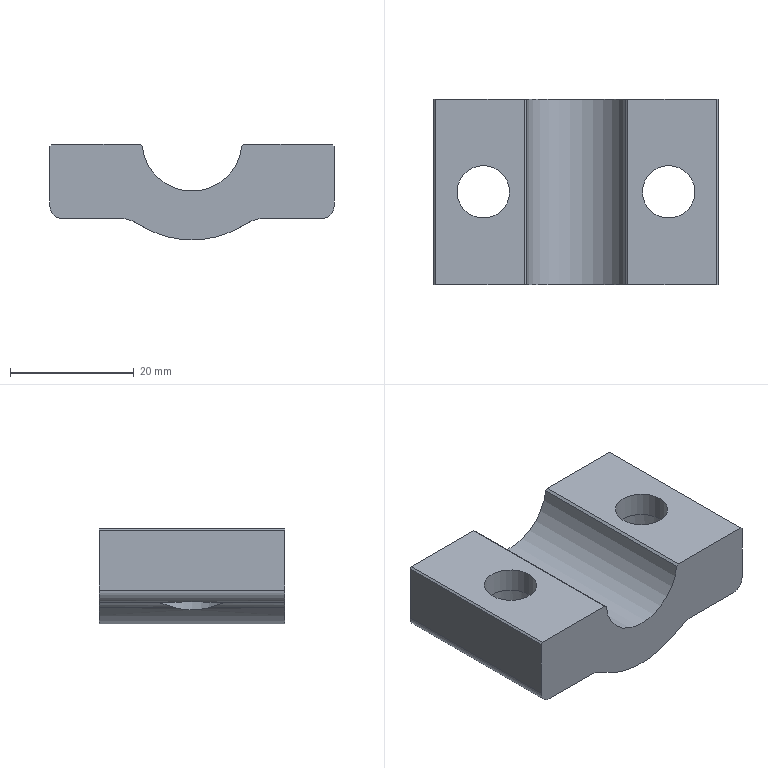Part | NX | 1 solid | 28 faces | box 46 x 30 x 15.5 mm | volume 12341 mm3 | plane 16 | cylinder 12 | commonest cylinder face diameters 10 x4 4 x2 8.5 x2 13.5 x2 16.2 x1 32 x1
STEP:
#1=CARTESIAN_POINT('',(14.61,0.,12.));
#2=VERTEX_POINT('',#1);
#3=CARTESIAN_POINT('',(0.3,0.,12.));
#4=VERTEX_POINT('',#3);
#5=CARTESIAN_POINT('',(23.,0.,12.));
#6=DIRECTION('',(-1.,0.,0.));
#7=VECTOR('',#6,1000.);
#8=LINE('',#5,#7);
#9=EDGE_CURVE('',#2,#4,#8,.T.);
#10=ORIENTED_EDGE('',*,*,#9,.F.);
#11=CARTESIAN_POINT('',(14.61,30.,12.));
#12=VERTEX_POINT('',#11);
#13=CARTESIAN_POINT('',(14.61,30.,12.));
#14=DIRECTION('',(0.,1.,0.));
#15=VECTOR('',#14,1000.);
#16=LINE('',#13,#15);
#17=EDGE_CURVE('',#2,#12,#16,.T.);
#18=ORIENTED_EDGE('',*,*,#17,.T.);
#19=CARTESIAN_POINT('',(0.3,30.,12.));
#20=VERTEX_POINT('',#19);
#21=CARTESIAN_POINT('',(23.,30.,12.));
#22=DIRECTION('',(1.,0.,0.));
#23=VECTOR('',#22,1000.);
#24=LINE('',#21,#23);
#25=EDGE_CURVE('',#20,#12,#24,.T.);
#26=ORIENTED_EDGE('',*,*,#25,.F.);
#27=CARTESIAN_POINT('',(0.3,15.,12.));
#28=DIRECTION('',(0.,-1.,0.));
#29=VECTOR('',#28,1000.);
#30=LINE('',#27,#29);
#31=EDGE_CURVE('',#20,#4,#30,.T.);
#32=ORIENTED_EDGE('',*,*,#31,.T.);
#33=EDGE_LOOP('',(#10,#18,#26,#32));
#34=FACE_BOUND('',#33,.T.);
#35=CARTESIAN_POINT('',(12.25,15.,12.));
#36=VERTEX_POINT('',#35);
#37=CARTESIAN_POINT('',(8.,15.,12.));
#38=DIRECTION('',(0.,0.,-1.));
#39=DIRECTION('',(1.,0.,0.));
#40=AXIS2_PLACEMENT_3D('',#37,#38,#39);
#41=CIRCLE('',#40,4.25);
#42=EDGE_CURVE('',#36,#36,#41,.T.);
#43=ORIENTED_EDGE('',*,*,#42,.T.);
#44=EDGE_LOOP('',(#43));
#45=FACE_BOUND('',#44,.T.);
#46=CARTESIAN_POINT('',(23.,15.,12.));
#47=DIRECTION('',(0.,0.,1.));
#48=DIRECTION('',(1.,0.,0.));
#49=AXIS2_PLACEMENT_3D('',#46,#47,#48);
#50=PLANE('',#49);
#51=ADVANCED_FACE('',(#34,#45),#50,.T.);
#52=CARTESIAN_POINT('',(34.608,0.,0.));
#53=VERTEX_POINT('',#52);
#54=CARTESIAN_POINT('',(34.608,9.164,0.));
#55=VERTEX_POINT('',#54);
#56=CARTESIAN_POINT('',(34.608,30.,0.));
#57=DIRECTION('',(0.,1.,0.));
#58=VECTOR('',#57,1000.);
#59=LINE('',#56,#58);
#60=EDGE_CURVE('',#53,#55,#59,.T.);
#61=ORIENTED_EDGE('',*,*,#60,.T.);
#62=CARTESIAN_POINT('',(44.,11.908,0.));
#63=VERTEX_POINT('',#62);
#64=CARTESIAN_POINT('',(38.,15.,0.));
#65=DIRECTION('',(0.,0.,-1.));
#66=DIRECTION('',(-1.,0.,0.));
#67=AXIS2_PLACEMENT_3D('',#64,#65,#66);
#68=CIRCLE('',#67,6.75);
#69=EDGE_CURVE('',#55,#63,#68,.F.);
#70=ORIENTED_EDGE('',*,*,#69,.T.);
#71=CARTESIAN_POINT('',(44.,0.,0.));
#72=VERTEX_POINT('',#71);
#73=CARTESIAN_POINT('',(44.,15.,0.));
#74=DIRECTION('',(0.,1.,0.));
#75=VECTOR('',#74,1000.);
#76=LINE('',#73,#75);
#77=EDGE_CURVE('',#63,#72,#76,.F.);
#78=ORIENTED_EDGE('',*,*,#77,.T.);
#79=CARTESIAN_POINT('',(23.,0.,0.));
#80=DIRECTION('',(1.,0.,0.));
#81=VECTOR('',#80,1000.);
#82=LINE('',#79,#81);
#83=EDGE_CURVE('',#53,#72,#82,.T.);
#84=ORIENTED_EDGE('',*,*,#83,.F.);
#85=EDGE_LOOP('',(#61,#70,#78,#84));
#86=FACE_BOUND('',#85,.T.);
#87=CARTESIAN_POINT('',(23.,15.,0.));
#88=DIRECTION('',(0.,0.,-1.));
#89=DIRECTION('',(-1.,0.,0.));
#90=AXIS2_PLACEMENT_3D('',#87,#88,#89);
#91=PLANE('',#90);
#92=ADVANCED_FACE('',(#86),#91,.T.);
#93=CARTESIAN_POINT('',(2.,0.,0.));
#94=VERTEX_POINT('',#93);
#95=CARTESIAN_POINT('',(2.,11.908,0.));
#96=VERTEX_POINT('',#95);
#97=CARTESIAN_POINT('',(2.,15.,0.));
#98=DIRECTION('',(0.,-1.,0.));
#99=VECTOR('',#98,1000.);
#100=LINE('',#97,#99);
#101=EDGE_CURVE('',#94,#96,#100,.F.);
#102=ORIENTED_EDGE('',*,*,#101,.T.);
#103=CARTESIAN_POINT('',(11.392,9.164,0.));
#104=VERTEX_POINT('',#103);
#105=CARTESIAN_POINT('',(8.,15.,0.));
#106=DIRECTION('',(0.,0.,-1.));
#107=DIRECTION('',(-1.,0.,0.));
#108=AXIS2_PLACEMENT_3D('',#105,#106,#107);
#109=CIRCLE('',#108,6.75);
#110=EDGE_CURVE('',#96,#104,#109,.F.);
#111=ORIENTED_EDGE('',*,*,#110,.T.);
#112=CARTESIAN_POINT('',(11.392,0.,0.));
#113=VERTEX_POINT('',#112);
#114=CARTESIAN_POINT('',(11.392,0.,0.));
#115=DIRECTION('',(0.,1.,0.));
#116=VECTOR('',#115,1000.);
#117=LINE('',#114,#116);
#118=EDGE_CURVE('',#104,#113,#117,.F.);
#119=ORIENTED_EDGE('',*,*,#118,.T.);
#120=CARTESIAN_POINT('',(23.,0.,0.));
#121=DIRECTION('',(1.,0.,0.));
#122=VECTOR('',#121,1000.);
#123=LINE('',#120,#122);
#124=EDGE_CURVE('',#94,#113,#123,.T.);
#125=ORIENTED_EDGE('',*,*,#124,.F.);
#126=EDGE_LOOP('',(#102,#111,#119,#125));
#127=FACE_BOUND('',#126,.T.);
#128=CARTESIAN_POINT('',(23.,15.,0.));
#129=DIRECTION('',(0.,0.,-1.));
#130=DIRECTION('',(-1.,0.,0.));
#131=AXIS2_PLACEMENT_3D('',#128,#129,#130);
#132=PLANE('',#131);
#133=ADVANCED_FACE('',(#127),#132,.T.);
#134=CARTESIAN_POINT('',(14.156,0.,-0.8333));
#135=VERTEX_POINT('',#134);
#136=CARTESIAN_POINT('',(14.156,12.23,-0.8333));
#137=VERTEX_POINT('',#136);
#138=CARTESIAN_POINT('',(14.156,30.,-0.8333));
#139=DIRECTION('',(0.,-1.,0.));
#140=VECTOR('',#139,1000.);
#141=LINE('',#138,#140);
#142=EDGE_CURVE('',#135,#137,#141,.F.);
#143=ORIENTED_EDGE('',*,*,#142,.T.);
#144=CARTESIAN_POINT('',(14.156,17.77,-0.8333));
#145=VERTEX_POINT('',#144);
#146=CARTESIAN_POINT('',(14.156,12.23,-0.8333));
#147=CARTESIAN_POINT('',(14.925,13.939,-1.343));
#148=CARTESIAN_POINT('',(14.925,16.061,-1.343));
#149=CARTESIAN_POINT('',(14.156,17.77,-0.8333));
#150=B_SPLINE_CURVE_WITH_KNOTS('',3,(#146,#147,#148,#149),.UNSPECIFIED.,.F.,.F.,(4,4),(0.,0.005745),.UNSPECIFIED.);
#151=EDGE_CURVE('',#137,#145,#150,.T.);
#152=ORIENTED_EDGE('',*,*,#151,.T.);
#153=CARTESIAN_POINT('',(14.156,30.,-0.8333));
#154=VERTEX_POINT('',#153);
#155=CARTESIAN_POINT('',(14.156,30.,-0.8333));
#156=DIRECTION('',(0.,-1.,0.));
#157=VECTOR('',#156,1000.);
#158=LINE('',#155,#157);
#159=EDGE_CURVE('',#145,#154,#158,.F.);
#160=ORIENTED_EDGE('',*,*,#159,.T.);
#161=CARTESIAN_POINT('',(31.844,30.,-0.8333));
#162=VERTEX_POINT('',#161);
#163=CARTESIAN_POINT('',(23.,30.,12.5));
#164=DIRECTION('',(0.,-1.,0.));
#165=DIRECTION('',(1.,0.,0.));
#166=AXIS2_PLACEMENT_3D('',#163,#164,#165);
#167=CIRCLE('',#166,16.);
#168=EDGE_CURVE('',#154,#162,#167,.T.);
#169=ORIENTED_EDGE('',*,*,#168,.T.);
#170=CARTESIAN_POINT('',(31.844,17.77,-0.8333));
#171=VERTEX_POINT('',#170);
#172=CARTESIAN_POINT('',(31.844,30.,-0.8333));
#173=DIRECTION('',(0.,-1.,0.));
#174=VECTOR('',#173,1000.);
#175=LINE('',#172,#174);
#176=EDGE_CURVE('',#162,#171,#175,.T.);
#177=ORIENTED_EDGE('',*,*,#176,.T.);
#178=CARTESIAN_POINT('',(31.844,12.23,-0.8333));
#179=VERTEX_POINT('',#178);
#180=CARTESIAN_POINT('',(31.844,17.77,-0.8333));
#181=CARTESIAN_POINT('',(31.075,16.061,-1.343));
#182=CARTESIAN_POINT('',(31.075,13.939,-1.343));
#183=CARTESIAN_POINT('',(31.844,12.23,-0.8333));
#184=B_SPLINE_CURVE_WITH_KNOTS('',3,(#180,#181,#182,#183),.UNSPECIFIED.,.F.,.F.,(4,4),(0.,0.005745),.UNSPECIFIED.);
#185=EDGE_CURVE('',#171,#179,#184,.T.);
#186=ORIENTED_EDGE('',*,*,#185,.T.);
#187=CARTESIAN_POINT('',(31.844,0.,-0.8333));
#188=VERTEX_POINT('',#187);
#189=CARTESIAN_POINT('',(31.844,30.,-0.8333));
#190=DIRECTION('',(0.,-1.,0.));
#191=VECTOR('',#190,1000.);
#192=LINE('',#189,#191);
#193=EDGE_CURVE('',#179,#188,#192,.T.);
#194=ORIENTED_EDGE('',*,*,#193,.T.);
#195=CARTESIAN_POINT('',(23.,0.,12.5));
#196=DIRECTION('',(0.,1.,0.));
#197=DIRECTION('',(1.,0.,0.));
#198=AXIS2_PLACEMENT_3D('',#195,#196,#197);
#199=CIRCLE('',#198,16.);
#200=EDGE_CURVE('',#188,#135,#199,.T.);
#201=ORIENTED_EDGE('',*,*,#200,.T.);
#202=EDGE_LOOP('',(#143,#152,#160,#169,#177,#186,#194,#201));
#203=FACE_BOUND('',#202,.T.);
#204=CARTESIAN_POINT('',(23.,30.,12.5));
#205=DIRECTION('',(0.,-1.,0.));
#206=DIRECTION('',(1.,0.,0.));
#207=AXIS2_PLACEMENT_3D('',#204,#205,#206);
#208=CYLINDRICAL_SURFACE('',#207,16.);
#209=ADVANCED_FACE('',(#203),#208,.T.);
#210=CARTESIAN_POINT('',(11.392,20.836,0.));
#211=VERTEX_POINT('',#210);
#212=CARTESIAN_POINT('',(11.392,20.836,0.));
#213=CARTESIAN_POINT('',(12.644,20.108,0.));
#214=CARTESIAN_POINT('',(13.585,19.039,-0.4545));
#215=CARTESIAN_POINT('',(14.156,17.77,-0.8333));
#216=B_SPLINE_CURVE_WITH_KNOTS('',3,(#212,#213,#214,#215),.UNSPECIFIED.,.F.,.F.,(4,4),(0.,0.004272),.UNSPECIFIED.);
#217=EDGE_CURVE('',#211,#145,#216,.T.);
#218=ORIENTED_EDGE('',*,*,#217,.F.);
#219=CARTESIAN_POINT('',(11.392,30.,0.));
#220=VERTEX_POINT('',#219);
#221=CARTESIAN_POINT('',(11.392,0.,0.));
#222=DIRECTION('',(0.,1.,0.));
#223=VECTOR('',#222,1000.);
#224=LINE('',#221,#223);
#225=EDGE_CURVE('',#220,#211,#224,.F.);
#226=ORIENTED_EDGE('',*,*,#225,.F.);
#227=CARTESIAN_POINT('',(11.392,30.,-5.));
#228=DIRECTION('',(0.,1.,0.));
#229=DIRECTION('',(0.,0.,1.));
#230=AXIS2_PLACEMENT_3D('',#227,#228,#229);
#231=CIRCLE('',#230,5.);
#232=EDGE_CURVE('',#154,#220,#231,.F.);
#233=ORIENTED_EDGE('',*,*,#232,.F.);
#234=ORIENTED_EDGE('',*,*,#159,.F.);
#235=EDGE_LOOP('',(#218,#226,#233,#234));
#236=FACE_BOUND('',#235,.T.);
#237=CARTESIAN_POINT('',(11.392,30.,-5.));
#238=DIRECTION('',(0.,-1.,0.));
#239=DIRECTION('',(0.,0.,-1.));
#240=AXIS2_PLACEMENT_3D('',#237,#238,#239);
#241=CYLINDRICAL_SURFACE('',#240,5.);
#242=ADVANCED_FACE('',(#236),#241,.F.);
#243=CARTESIAN_POINT('',(14.156,12.23,-0.8333));
#244=CARTESIAN_POINT('',(13.585,10.961,-0.4545));
#245=CARTESIAN_POINT('',(12.644,9.892,0.));
#246=CARTESIAN_POINT('',(11.392,9.164,0.));
#247=B_SPLINE_CURVE_WITH_KNOTS('',3,(#243,#244,#245,#246),.UNSPECIFIED.,.F.,.F.,(4,4),(0.,0.00426),.UNSPECIFIED.);
#248=EDGE_CURVE('',#137,#104,#247,.T.);
#249=ORIENTED_EDGE('',*,*,#248,.F.);
#250=ORIENTED_EDGE('',*,*,#142,.F.);
#251=CARTESIAN_POINT('',(11.392,0.,-5.));
#252=DIRECTION('',(0.,-1.,0.));
#253=DIRECTION('',(0.,0.,-1.));
#254=AXIS2_PLACEMENT_3D('',#251,#252,#253);
#255=CIRCLE('',#254,5.);
#256=EDGE_CURVE('',#113,#135,#255,.F.);
#257=ORIENTED_EDGE('',*,*,#256,.F.);
#258=ORIENTED_EDGE('',*,*,#118,.F.);
#259=EDGE_LOOP('',(#249,#250,#257,#258));
#260=FACE_BOUND('',#259,.T.);
#261=CARTESIAN_POINT('',(11.392,30.,-5.));
#262=DIRECTION('',(0.,-1.,0.));
#263=DIRECTION('',(0.,0.,-1.));
#264=AXIS2_PLACEMENT_3D('',#261,#262,#263);
#265=CYLINDRICAL_SURFACE('',#264,5.);
#266=ADVANCED_FACE('',(#260),#265,.F.);
#267=CARTESIAN_POINT('',(34.608,20.836,0.));
#268=VERTEX_POINT('',#267);
#269=CARTESIAN_POINT('',(31.844,17.77,-0.8333));
#270=CARTESIAN_POINT('',(32.415,19.039,-0.4545));
#271=CARTESIAN_POINT('',(33.356,20.108,0.));
#272=CARTESIAN_POINT('',(34.608,20.836,0.));
#273=B_SPLINE_CURVE_WITH_KNOTS('',3,(#269,#270,#271,#272),.UNSPECIFIED.,.F.,.F.,(4,4),(0.,0.00426),.UNSPECIFIED.);
#274=EDGE_CURVE('',#171,#268,#273,.T.);
#275=ORIENTED_EDGE('',*,*,#274,.F.);
#276=ORIENTED_EDGE('',*,*,#176,.F.);
#277=CARTESIAN_POINT('',(34.608,30.,0.));
#278=VERTEX_POINT('',#277);
#279=CARTESIAN_POINT('',(34.608,30.,-5.));
#280=DIRECTION('',(0.,1.,0.));
#281=DIRECTION('',(0.,0.,1.));
#282=AXIS2_PLACEMENT_3D('',#279,#280,#281);
#283=CIRCLE('',#282,5.);
#284=EDGE_CURVE('',#278,#162,#283,.F.);
#285=ORIENTED_EDGE('',*,*,#284,.F.);
#286=CARTESIAN_POINT('',(34.608,30.,0.));
#287=DIRECTION('',(0.,1.,0.));
#288=VECTOR('',#287,1000.);
#289=LINE('',#286,#288);
#290=EDGE_CURVE('',#268,#278,#289,.T.);
#291=ORIENTED_EDGE('',*,*,#290,.F.);
#292=EDGE_LOOP('',(#275,#276,#285,#291));
#293=FACE_BOUND('',#292,.T.);
#294=CARTESIAN_POINT('',(34.608,30.,-5.));
#295=DIRECTION('',(0.,-1.,0.));
#296=DIRECTION('',(0.,0.,-1.));
#297=AXIS2_PLACEMENT_3D('',#294,#295,#296);
#298=CYLINDRICAL_SURFACE('',#297,5.);
#299=ADVANCED_FACE('',(#293),#298,.F.);
#300=CARTESIAN_POINT('',(34.608,9.164,0.));
#301=CARTESIAN_POINT('',(33.356,9.892,0.));
#302=CARTESIAN_POINT('',(32.415,10.961,-0.4545));
#303=CARTESIAN_POINT('',(31.844,12.23,-0.8333));
#304=B_SPLINE_CURVE_WITH_KNOTS('',3,(#300,#301,#302,#303),.UNSPECIFIED.,.F.,.F.,(4,4),(0.,0.004272),.UNSPECIFIED.);
#305=EDGE_CURVE('',#55,#179,#304,.T.);
#306=ORIENTED_EDGE('',*,*,#305,.F.);
#307=ORIENTED_EDGE('',*,*,#60,.F.);
#308=CARTESIAN_POINT('',(34.608,0.,-5.));
#309=DIRECTION('',(0.,-1.,0.));
#310=DIRECTION('',(0.,0.,-1.));
#311=AXIS2_PLACEMENT_3D('',#308,#309,#310);
#312=CIRCLE('',#311,5.);
#313=EDGE_CURVE('',#188,#53,#312,.F.);
#314=ORIENTED_EDGE('',*,*,#313,.F.);
#315=ORIENTED_EDGE('',*,*,#193,.F.);
#316=EDGE_LOOP('',(#306,#307,#314,#315));
#317=FACE_BOUND('',#316,.T.);
#318=CARTESIAN_POINT('',(34.608,30.,-5.));
#319=DIRECTION('',(0.,-1.,0.));
#320=DIRECTION('',(0.,0.,-1.));
#321=AXIS2_PLACEMENT_3D('',#318,#319,#320);
#322=CYLINDRICAL_SURFACE('',#321,5.);
#323=ADVANCED_FACE('',(#317),#322,.F.);
#324=ORIENTED_EDGE('',*,*,#77,.F.);
#325=CARTESIAN_POINT('',(44.,18.092,0.));
#326=VERTEX_POINT('',#325);
#327=CARTESIAN_POINT('',(44.,11.908,0.));
#328=CARTESIAN_POINT('',(44.496,12.87,0.));
#329=CARTESIAN_POINT('',(45.004,15.001,0.2919));
#330=CARTESIAN_POINT('',(44.496,17.13,0.));
#331=CARTESIAN_POINT('',(44.,18.092,0.));
#332=B_SPLINE_CURVE_WITH_KNOTS('',3,(#327,#328,#329,#330,#331),.UNSPECIFIED.,.F.,.F.,(4,1,4),(0.,0.003207,0.006415),.UNSPECIFIED.);
#333=EDGE_CURVE('',#63,#326,#332,.T.);
#334=ORIENTED_EDGE('',*,*,#333,.T.);
#335=CARTESIAN_POINT('',(44.,30.,0.));
#336=VERTEX_POINT('',#335);
#337=CARTESIAN_POINT('',(44.,15.,0.));
#338=DIRECTION('',(0.,1.,0.));
#339=VECTOR('',#338,1000.);
#340=LINE('',#337,#339);
#341=EDGE_CURVE('',#336,#326,#340,.F.);
#342=ORIENTED_EDGE('',*,*,#341,.F.);
#343=CARTESIAN_POINT('',(46.,30.,2.));
#344=VERTEX_POINT('',#343);
#345=CARTESIAN_POINT('',(44.,30.,2.));
#346=DIRECTION('',(0.,1.,0.));
#347=DIRECTION('',(0.,0.,1.));
#348=AXIS2_PLACEMENT_3D('',#345,#346,#347);
#349=CIRCLE('',#348,2.);
#350=EDGE_CURVE('',#344,#336,#349,.T.);
#351=ORIENTED_EDGE('',*,*,#350,.F.);
#352=CARTESIAN_POINT('',(46.,0.,2.));
#353=VERTEX_POINT('',#352);
#354=CARTESIAN_POINT('',(46.,15.,2.));
#355=DIRECTION('',(0.,1.,0.));
#356=VECTOR('',#355,1000.);
#357=LINE('',#354,#356);
#358=EDGE_CURVE('',#353,#344,#357,.T.);
#359=ORIENTED_EDGE('',*,*,#358,.F.);
#360=CARTESIAN_POINT('',(44.,0.,2.));
#361=DIRECTION('',(0.,-1.,0.));
#362=DIRECTION('',(0.,0.,-1.));
#363=AXIS2_PLACEMENT_3D('',#360,#361,#362);
#364=CIRCLE('',#363,2.);
#365=EDGE_CURVE('',#72,#353,#364,.T.);
#366=ORIENTED_EDGE('',*,*,#365,.F.);
#367=EDGE_LOOP('',(#324,#334,#342,#351,#359,#366));
#368=FACE_BOUND('',#367,.T.);
#369=CARTESIAN_POINT('',(44.,15.,2.));
#370=DIRECTION('',(0.,1.,0.));
#371=DIRECTION('',(0.,0.,1.));
#372=AXIS2_PLACEMENT_3D('',#369,#370,#371);
#373=CYLINDRICAL_SURFACE('',#372,2.);
#374=ADVANCED_FACE('',(#368),#373,.T.);
#375=CARTESIAN_POINT('',(2.,18.092,0.));
#376=VERTEX_POINT('',#375);
#377=CARTESIAN_POINT('',(2.,30.,0.));
#378=VERTEX_POINT('',#377);
#379=CARTESIAN_POINT('',(2.,15.,0.));
#380=DIRECTION('',(0.,-1.,0.));
#381=VECTOR('',#380,1000.);
#382=LINE('',#379,#381);
#383=EDGE_CURVE('',#376,#378,#382,.F.);
#384=ORIENTED_EDGE('',*,*,#383,.F.);
#385=CARTESIAN_POINT('',(2.,18.092,0.));
#386=CARTESIAN_POINT('',(1.504,17.13,0.));
#387=CARTESIAN_POINT('',(0.9961,14.999,0.2919));
#388=CARTESIAN_POINT('',(1.504,12.87,0.));
#389=CARTESIAN_POINT('',(2.,11.908,0.));
#390=B_SPLINE_CURVE_WITH_KNOTS('',3,(#385,#386,#387,#388,#389),.UNSPECIFIED.,.F.,.F.,(4,1,4),(0.,0.003207,0.006415),.UNSPECIFIED.);
#391=EDGE_CURVE('',#376,#96,#390,.T.);
#392=ORIENTED_EDGE('',*,*,#391,.T.);
#393=ORIENTED_EDGE('',*,*,#101,.F.);
#394=CARTESIAN_POINT('',(0.,0.,2.));
#395=VERTEX_POINT('',#394);
#396=CARTESIAN_POINT('',(2.,0.,2.));
#397=DIRECTION('',(0.,-1.,0.));
#398=DIRECTION('',(0.,0.,-1.));
#399=AXIS2_PLACEMENT_3D('',#396,#397,#398);
#400=CIRCLE('',#399,2.);
#401=EDGE_CURVE('',#395,#94,#400,.T.);
#402=ORIENTED_EDGE('',*,*,#401,.F.);
#403=CARTESIAN_POINT('',(0.,30.,2.));
#404=VERTEX_POINT('',#403);
#405=CARTESIAN_POINT('',(0.,15.,2.));
#406=DIRECTION('',(0.,-1.,0.));
#407=VECTOR('',#406,1000.);
#408=LINE('',#405,#407);
#409=EDGE_CURVE('',#404,#395,#408,.T.);
#410=ORIENTED_EDGE('',*,*,#409,.F.);
#411=CARTESIAN_POINT('',(2.,30.,2.));
#412=DIRECTION('',(0.,1.,0.));
#413=DIRECTION('',(0.,0.,1.));
#414=AXIS2_PLACEMENT_3D('',#411,#412,#413);
#415=CIRCLE('',#414,2.);
#416=EDGE_CURVE('',#378,#404,#415,.T.);
#417=ORIENTED_EDGE('',*,*,#416,.F.);
#418=EDGE_LOOP('',(#384,#392,#393,#402,#410,#417));
#419=FACE_BOUND('',#418,.T.);
#420=CARTESIAN_POINT('',(2.,15.,2.));
#421=DIRECTION('',(0.,-1.,0.));
#422=DIRECTION('',(0.,0.,-1.));
#423=AXIS2_PLACEMENT_3D('',#420,#421,#422);
#424=CYLINDRICAL_SURFACE('',#423,2.);
#425=ADVANCED_FACE('',(#419),#424,.T.);
#426=CARTESIAN_POINT('',(42.25,15.,12.));
#427=VERTEX_POINT('',#426);
#428=CARTESIAN_POINT('',(38.,15.,12.));
#429=DIRECTION('',(0.,0.,-1.));
#430=DIRECTION('',(1.,0.,0.));
#431=AXIS2_PLACEMENT_3D('',#428,#429,#430);
#432=CIRCLE('',#431,4.25);
#433=EDGE_CURVE('',#427,#427,#432,.T.);
#434=ORIENTED_EDGE('',*,*,#433,.F.);
#435=EDGE_LOOP('',(#434));
#436=FACE_BOUND('',#435,.T.);
#437=CARTESIAN_POINT('',(33.75,15.,8.));
#438=VERTEX_POINT('',#437);
#439=CARTESIAN_POINT('',(38.,15.,8.));
#440=DIRECTION('',(0.,0.,-1.));
#441=DIRECTION('',(-1.,0.,0.));
#442=AXIS2_PLACEMENT_3D('',#439,#440,#441);
#443=CIRCLE('',#442,4.25);
#444=EDGE_CURVE('',#438,#438,#443,.F.);
#445=ORIENTED_EDGE('',*,*,#444,.F.);
#446=EDGE_LOOP('',(#445));
#447=FACE_BOUND('',#446,.T.);
#448=CARTESIAN_POINT('',(38.,15.,12.));
#449=DIRECTION('',(0.,0.,-1.));
#450=DIRECTION('',(1.,0.,0.));
#451=AXIS2_PLACEMENT_3D('',#448,#449,#450);
#452=CYLINDRICAL_SURFACE('',#451,4.25);
#453=ADVANCED_FACE('',(#436,#447),#452,.F.);
#454=ORIENTED_EDGE('',*,*,#42,.F.);
#455=EDGE_LOOP('',(#454));
#456=FACE_BOUND('',#455,.T.);
#457=CARTESIAN_POINT('',(3.75,15.,8.));
#458=VERTEX_POINT('',#457);
#459=CARTESIAN_POINT('',(8.,15.,8.));
#460=DIRECTION('',(0.,0.,-1.));
#461=DIRECTION('',(-1.,0.,0.));
#462=AXIS2_PLACEMENT_3D('',#459,#460,#461);
#463=CIRCLE('',#462,4.25);
#464=EDGE_CURVE('',#458,#458,#463,.F.);
#465=ORIENTED_EDGE('',*,*,#464,.F.);
#466=EDGE_LOOP('',(#465));
#467=FACE_BOUND('',#466,.T.);
#468=CARTESIAN_POINT('',(8.,15.,12.));
#469=DIRECTION('',(0.,0.,-1.));
#470=DIRECTION('',(1.,0.,0.));
#471=AXIS2_PLACEMENT_3D('',#468,#469,#470);
#472=CYLINDRICAL_SURFACE('',#471,4.25);
#473=ADVANCED_FACE('',(#456,#467),#472,.F.);
#474=ORIENTED_EDGE('',*,*,#341,.T.);
#475=CARTESIAN_POINT('',(38.,15.,0.));
#476=DIRECTION('',(0.,0.,-1.));
#477=DIRECTION('',(-1.,0.,0.));
#478=AXIS2_PLACEMENT_3D('',#475,#476,#477);
#479=CIRCLE('',#478,6.75);
#480=EDGE_CURVE('',#326,#268,#479,.F.);
#481=ORIENTED_EDGE('',*,*,#480,.T.);
#482=ORIENTED_EDGE('',*,*,#290,.T.);
#483=CARTESIAN_POINT('',(23.,30.,0.));
#484=DIRECTION('',(-1.,0.,0.));
#485=VECTOR('',#484,1000.);
#486=LINE('',#483,#485);
#487=EDGE_CURVE('',#336,#278,#486,.T.);
#488=ORIENTED_EDGE('',*,*,#487,.F.);
#489=EDGE_LOOP('',(#474,#481,#482,#488));
#490=FACE_BOUND('',#489,.T.);
#491=CARTESIAN_POINT('',(23.,15.,0.));
#492=DIRECTION('',(0.,0.,-1.));
#493=DIRECTION('',(-1.,0.,0.));
#494=AXIS2_PLACEMENT_3D('',#491,#492,#493);
#495=PLANE('',#494);
#496=ADVANCED_FACE('',(#490),#495,.T.);
#497=CARTESIAN_POINT('',(45.7,0.,12.));
#498=VERTEX_POINT('',#497);
#499=CARTESIAN_POINT('',(31.39,0.,12.));
#500=VERTEX_POINT('',#499);
#501=CARTESIAN_POINT('',(23.,0.,12.));
#502=DIRECTION('',(-1.,0.,0.));
#503=VECTOR('',#502,1000.);
#504=LINE('',#501,#503);
#505=EDGE_CURVE('',#498,#500,#504,.T.);
#506=ORIENTED_EDGE('',*,*,#505,.F.);
#507=CARTESIAN_POINT('',(45.7,30.,12.));
#508=VERTEX_POINT('',#507);
#509=CARTESIAN_POINT('',(45.7,15.,12.));
#510=DIRECTION('',(0.,1.,0.));
#511=VECTOR('',#510,1000.);
#512=LINE('',#509,#511);
#513=EDGE_CURVE('',#498,#508,#512,.T.);
#514=ORIENTED_EDGE('',*,*,#513,.T.);
#515=CARTESIAN_POINT('',(31.39,30.,12.));
#516=VERTEX_POINT('',#515);
#517=CARTESIAN_POINT('',(23.,30.,12.));
#518=DIRECTION('',(1.,0.,0.));
#519=VECTOR('',#518,1000.);
#520=LINE('',#517,#519);
#521=EDGE_CURVE('',#516,#508,#520,.T.);
#522=ORIENTED_EDGE('',*,*,#521,.F.);
#523=CARTESIAN_POINT('',(31.39,0.,12.));
#524=DIRECTION('',(0.,-1.,0.));
#525=VECTOR('',#524,1000.);
#526=LINE('',#523,#525);
#527=EDGE_CURVE('',#516,#500,#526,.T.);
#528=ORIENTED_EDGE('',*,*,#527,.T.);
#529=EDGE_LOOP('',(#506,#514,#522,#528));
#530=FACE_BOUND('',#529,.T.);
#531=ORIENTED_EDGE('',*,*,#433,.T.);
#532=EDGE_LOOP('',(#531));
#533=FACE_BOUND('',#532,.T.);
#534=CARTESIAN_POINT('',(23.,15.,12.));
#535=DIRECTION('',(0.,0.,1.));
#536=DIRECTION('',(1.,0.,0.));
#537=AXIS2_PLACEMENT_3D('',#534,#535,#536);
#538=PLANE('',#537);
#539=ADVANCED_FACE('',(#530,#533),#538,.T.);
#540=CARTESIAN_POINT('',(46.,0.,11.7));
#541=VERTEX_POINT('',#540);
#542=CARTESIAN_POINT('',(46.,0.,0.));
#543=DIRECTION('',(0.,0.,1.));
#544=VECTOR('',#543,1000.);
#545=LINE('',#542,#544);
#546=EDGE_CURVE('',#353,#541,#545,.T.);
#547=ORIENTED_EDGE('',*,*,#546,.T.);
#548=CARTESIAN_POINT('',(40.35,0.,17.35));
#549=DIRECTION('',(0.7071,0.,-0.7071));
#550=VECTOR('',#549,1000.);
#551=LINE('',#548,#550);
#552=EDGE_CURVE('',#541,#498,#551,.F.);
#553=ORIENTED_EDGE('',*,*,#552,.T.);
#554=ORIENTED_EDGE('',*,*,#505,.T.);
#555=CARTESIAN_POINT('',(31.061,0.,11.701));
#556=VERTEX_POINT('',#555);
#557=CARTESIAN_POINT('',(20.811,0.,2.417));
#558=DIRECTION('',(-0.7411,0.,-0.6713));
#559=VECTOR('',#558,1000.);
#560=LINE('',#557,#559);
#561=EDGE_CURVE('',#500,#556,#560,.T.);
#562=ORIENTED_EDGE('',*,*,#561,.T.);
#563=CARTESIAN_POINT('',(14.939,0.,11.701));
#564=VERTEX_POINT('',#563);
#565=CARTESIAN_POINT('',(23.,0.,12.5));
#566=DIRECTION('',(0.,1.,0.));
#567=DIRECTION('',(1.,0.,0.));
#568=AXIS2_PLACEMENT_3D('',#565,#566,#567);
#569=CIRCLE('',#568,8.1);
#570=EDGE_CURVE('',#556,#564,#569,.T.);
#571=ORIENTED_EDGE('',*,*,#570,.T.);
#572=CARTESIAN_POINT('',(25.189,0.,2.417));
#573=DIRECTION('',(0.7411,0.,-0.6713));
#574=VECTOR('',#573,1000.);
#575=LINE('',#572,#574);
#576=EDGE_CURVE('',#564,#2,#575,.F.);
#577=ORIENTED_EDGE('',*,*,#576,.T.);
#578=ORIENTED_EDGE('',*,*,#9,.T.);
#579=CARTESIAN_POINT('',(0.,0.,11.7));
#580=VERTEX_POINT('',#579);
#581=CARTESIAN_POINT('',(5.65,0.,17.35));
#582=DIRECTION('',(0.7071,0.,0.7071));
#583=VECTOR('',#582,1000.);
#584=LINE('',#581,#583);
#585=EDGE_CURVE('',#4,#580,#584,.F.);
#586=ORIENTED_EDGE('',*,*,#585,.T.);
#587=CARTESIAN_POINT('',(0.,0.,0.));
#588=DIRECTION('',(0.,0.,1.));
#589=VECTOR('',#588,1000.);
#590=LINE('',#587,#589);
#591=EDGE_CURVE('',#395,#580,#590,.T.);
#592=ORIENTED_EDGE('',*,*,#591,.F.);
#593=ORIENTED_EDGE('',*,*,#401,.T.);
#594=ORIENTED_EDGE('',*,*,#124,.T.);
#595=ORIENTED_EDGE('',*,*,#256,.T.);
#596=ORIENTED_EDGE('',*,*,#200,.F.);
#597=ORIENTED_EDGE('',*,*,#313,.T.);
#598=ORIENTED_EDGE('',*,*,#83,.T.);
#599=ORIENTED_EDGE('',*,*,#365,.T.);
#600=EDGE_LOOP('',(#547,#553,#554,#562,#571,#577,#578,#586,#592,#593,#594,#595,#596,#597,#598,#599));
#601=FACE_BOUND('',#600,.T.);
#602=CARTESIAN_POINT('',(23.,0.,0.));
#603=DIRECTION('',(0.,-1.,0.));
#604=DIRECTION('',(0.,0.,-1.));
#605=AXIS2_PLACEMENT_3D('',#602,#603,#604);
#606=PLANE('',#605);
#607=ADVANCED_FACE('',(#601),#606,.T.);
#608=ORIENTED_EDGE('',*,*,#591,.T.);
#609=CARTESIAN_POINT('',(0.,30.,11.7));
#610=VERTEX_POINT('',#609);
#611=CARTESIAN_POINT('',(0.,15.,11.7));
#612=DIRECTION('',(0.,1.,0.));
#613=VECTOR('',#612,1000.);
#614=LINE('',#611,#613);
#615=EDGE_CURVE('',#580,#610,#614,.T.);
#616=ORIENTED_EDGE('',*,*,#615,.T.);
#617=CARTESIAN_POINT('',(0.,30.,0.));
#618=DIRECTION('',(0.,0.,1.));
#619=VECTOR('',#618,1000.);
#620=LINE('',#617,#619);
#621=EDGE_CURVE('',#404,#610,#620,.T.);
#622=ORIENTED_EDGE('',*,*,#621,.F.);
#623=ORIENTED_EDGE('',*,*,#409,.T.);
#624=EDGE_LOOP('',(#608,#616,#622,#623));
#625=FACE_BOUND('',#624,.T.);
#626=CARTESIAN_POINT('',(0.,15.,0.));
#627=DIRECTION('',(-1.,0.,0.));
#628=DIRECTION('',(0.,0.,1.));
#629=AXIS2_PLACEMENT_3D('',#626,#627,#628);
#630=PLANE('',#629);
#631=ADVANCED_FACE('',(#625),#630,.T.);
#632=ORIENTED_EDGE('',*,*,#521,.T.);
#633=CARTESIAN_POINT('',(46.,30.,11.7));
#634=VERTEX_POINT('',#633);
#635=CARTESIAN_POINT('',(40.35,30.,17.35));
#636=DIRECTION('',(-0.7071,0.,0.7071));
#637=VECTOR('',#636,1000.);
#638=LINE('',#635,#637);
#639=EDGE_CURVE('',#508,#634,#638,.F.);
#640=ORIENTED_EDGE('',*,*,#639,.T.);
#641=CARTESIAN_POINT('',(46.,30.,0.));
#642=DIRECTION('',(0.,0.,1.));
#643=VECTOR('',#642,1000.);
#644=LINE('',#641,#643);
#645=EDGE_CURVE('',#344,#634,#644,.T.);
#646=ORIENTED_EDGE('',*,*,#645,.F.);
#647=ORIENTED_EDGE('',*,*,#350,.T.);
#648=ORIENTED_EDGE('',*,*,#487,.T.);
#649=ORIENTED_EDGE('',*,*,#284,.T.);
#650=ORIENTED_EDGE('',*,*,#168,.F.);
#651=ORIENTED_EDGE('',*,*,#232,.T.);
#652=CARTESIAN_POINT('',(23.,30.,0.));
#653=DIRECTION('',(-1.,0.,0.));
#654=VECTOR('',#653,1000.);
#655=LINE('',#652,#654);
#656=EDGE_CURVE('',#220,#378,#655,.T.);
#657=ORIENTED_EDGE('',*,*,#656,.T.);
#658=ORIENTED_EDGE('',*,*,#416,.T.);
#659=ORIENTED_EDGE('',*,*,#621,.T.);
#660=CARTESIAN_POINT('',(5.65,30.,17.35));
#661=DIRECTION('',(-0.7071,0.,-0.7071));
#662=VECTOR('',#661,1000.);
#663=LINE('',#660,#662);
#664=EDGE_CURVE('',#610,#20,#663,.F.);
#665=ORIENTED_EDGE('',*,*,#664,.T.);
#666=ORIENTED_EDGE('',*,*,#25,.T.);
#667=CARTESIAN_POINT('',(14.939,30.,11.701));
#668=VERTEX_POINT('',#667);
#669=CARTESIAN_POINT('',(25.189,30.,2.417));
#670=DIRECTION('',(-0.7411,0.,0.6713));
#671=VECTOR('',#670,1000.);
#672=LINE('',#669,#671);
#673=EDGE_CURVE('',#12,#668,#672,.F.);
#674=ORIENTED_EDGE('',*,*,#673,.T.);
#675=CARTESIAN_POINT('',(31.061,30.,11.701));
#676=VERTEX_POINT('',#675);
#677=CARTESIAN_POINT('',(23.,30.,12.5));
#678=DIRECTION('',(0.,-1.,0.));
#679=DIRECTION('',(1.,0.,0.));
#680=AXIS2_PLACEMENT_3D('',#677,#678,#679);
#681=CIRCLE('',#680,8.1);
#682=EDGE_CURVE('',#668,#676,#681,.T.);
#683=ORIENTED_EDGE('',*,*,#682,.T.);
#684=CARTESIAN_POINT('',(20.811,30.,2.417));
#685=DIRECTION('',(0.7411,0.,0.6713));
#686=VECTOR('',#685,1000.);
#687=LINE('',#684,#686);
#688=EDGE_CURVE('',#676,#516,#687,.T.);
#689=ORIENTED_EDGE('',*,*,#688,.T.);
#690=EDGE_LOOP('',(#632,#640,#646,#647,#648,#649,#650,#651,#657,#658,#659,#665,#666,#674,#683,#689));
#691=FACE_BOUND('',#690,.T.);
#692=CARTESIAN_POINT('',(23.,30.,0.));
#693=DIRECTION('',(0.,1.,0.));
#694=DIRECTION('',(0.,0.,1.));
#695=AXIS2_PLACEMENT_3D('',#692,#693,#694);
#696=PLANE('',#695);
#697=ADVANCED_FACE('',(#691),#696,.T.);
#698=ORIENTED_EDGE('',*,*,#225,.T.);
#699=CARTESIAN_POINT('',(8.,15.,0.));
#700=DIRECTION('',(0.,0.,-1.));
#701=DIRECTION('',(-1.,0.,0.));
#702=AXIS2_PLACEMENT_3D('',#699,#700,#701);
#703=CIRCLE('',#702,6.75);
#704=EDGE_CURVE('',#211,#376,#703,.F.);
#705=ORIENTED_EDGE('',*,*,#704,.T.);
#706=ORIENTED_EDGE('',*,*,#383,.T.);
#707=ORIENTED_EDGE('',*,*,#656,.F.);
#708=EDGE_LOOP('',(#698,#705,#706,#707));
#709=FACE_BOUND('',#708,.T.);
#710=CARTESIAN_POINT('',(23.,15.,0.));
#711=DIRECTION('',(0.,0.,-1.));
#712=DIRECTION('',(-1.,0.,0.));
#713=AXIS2_PLACEMENT_3D('',#710,#711,#712);
#714=PLANE('',#713);
#715=ADVANCED_FACE('',(#709),#714,.T.);
#716=ORIENTED_EDGE('',*,*,#645,.T.);
#717=CARTESIAN_POINT('',(46.,15.,11.7));
#718=DIRECTION('',(0.,-1.,0.));
#719=VECTOR('',#718,1000.);
#720=LINE('',#717,#719);
#721=EDGE_CURVE('',#634,#541,#720,.T.);
#722=ORIENTED_EDGE('',*,*,#721,.T.);
#723=ORIENTED_EDGE('',*,*,#546,.F.);
#724=ORIENTED_EDGE('',*,*,#358,.T.);
#725=EDGE_LOOP('',(#716,#722,#723,#724));
#726=FACE_BOUND('',#725,.T.);
#727=CARTESIAN_POINT('',(46.,15.,0.));
#728=DIRECTION('',(1.,0.,0.));
#729=DIRECTION('',(0.,0.,-1.));
#730=AXIS2_PLACEMENT_3D('',#727,#728,#729);
#731=PLANE('',#730);
#732=ADVANCED_FACE('',(#726),#731,.T.);
#733=CARTESIAN_POINT('',(1.25,15.,8.));
#734=VERTEX_POINT('',#733);
#735=CARTESIAN_POINT('',(8.,15.,8.));
#736=DIRECTION('',(0.,0.,-1.));
#737=DIRECTION('',(-1.,0.,0.));
#738=AXIS2_PLACEMENT_3D('',#735,#736,#737);
#739=CIRCLE('',#738,6.75);
#740=EDGE_CURVE('',#734,#734,#739,.F.);
#741=ORIENTED_EDGE('',*,*,#740,.F.);
#742=EDGE_LOOP('',(#741));
#743=FACE_BOUND('',#742,.T.);
#744=ORIENTED_EDGE('',*,*,#464,.T.);
#745=EDGE_LOOP('',(#744));
#746=FACE_BOUND('',#745,.T.);
#747=CARTESIAN_POINT('',(8.,15.,8.));
#748=DIRECTION('',(0.,0.,-1.));
#749=DIRECTION('',(-1.,0.,0.));
#750=AXIS2_PLACEMENT_3D('',#747,#748,#749);
#751=PLANE('',#750);
#752=ADVANCED_FACE('',(#743,#746),#751,.T.);
#753=ORIENTED_EDGE('',*,*,#248,.T.);
#754=ORIENTED_EDGE('',*,*,#110,.F.);
#755=ORIENTED_EDGE('',*,*,#391,.F.);
#756=ORIENTED_EDGE('',*,*,#704,.F.);
#757=ORIENTED_EDGE('',*,*,#217,.T.);
#758=ORIENTED_EDGE('',*,*,#151,.F.);
#759=EDGE_LOOP('',(#753,#754,#755,#756,#757,#758));
#760=FACE_BOUND('',#759,.T.);
#761=ORIENTED_EDGE('',*,*,#740,.T.);
#762=EDGE_LOOP('',(#761));
#763=FACE_BOUND('',#762,.T.);
#764=CARTESIAN_POINT('',(8.,15.,-13.));
#765=DIRECTION('',(0.,0.,1.));
#766=DIRECTION('',(1.,0.,0.));
#767=AXIS2_PLACEMENT_3D('',#764,#765,#766);
#768=CYLINDRICAL_SURFACE('',#767,6.75);
#769=ADVANCED_FACE('',(#760,#763),#768,.F.);
#770=CARTESIAN_POINT('',(31.25,15.,8.));
#771=VERTEX_POINT('',#770);
#772=CARTESIAN_POINT('',(38.,15.,8.));
#773=DIRECTION('',(0.,0.,-1.));
#774=DIRECTION('',(-1.,0.,0.));
#775=AXIS2_PLACEMENT_3D('',#772,#773,#774);
#776=CIRCLE('',#775,6.75);
#777=EDGE_CURVE('',#771,#771,#776,.F.);
#778=ORIENTED_EDGE('',*,*,#777,.F.);
#779=EDGE_LOOP('',(#778));
#780=FACE_BOUND('',#779,.T.);
#781=ORIENTED_EDGE('',*,*,#444,.T.);
#782=EDGE_LOOP('',(#781));
#783=FACE_BOUND('',#782,.T.);
#784=CARTESIAN_POINT('',(38.,15.,8.));
#785=DIRECTION('',(0.,0.,-1.));
#786=DIRECTION('',(-1.,0.,0.));
#787=AXIS2_PLACEMENT_3D('',#784,#785,#786);
#788=PLANE('',#787);
#789=ADVANCED_FACE('',(#780,#783),#788,.T.);
#790=ORIENTED_EDGE('',*,*,#274,.T.);
#791=ORIENTED_EDGE('',*,*,#480,.F.);
#792=ORIENTED_EDGE('',*,*,#333,.F.);
#793=ORIENTED_EDGE('',*,*,#69,.F.);
#794=ORIENTED_EDGE('',*,*,#305,.T.);
#795=ORIENTED_EDGE('',*,*,#185,.F.);
#796=EDGE_LOOP('',(#790,#791,#792,#793,#794,#795));
#797=FACE_BOUND('',#796,.T.);
#798=ORIENTED_EDGE('',*,*,#777,.T.);
#799=EDGE_LOOP('',(#798));
#800=FACE_BOUND('',#799,.T.);
#801=CARTESIAN_POINT('',(38.,15.,-13.));
#802=DIRECTION('',(0.,0.,1.));
#803=DIRECTION('',(1.,0.,0.));
#804=AXIS2_PLACEMENT_3D('',#801,#802,#803);
#805=CYLINDRICAL_SURFACE('',#804,6.75);
#806=ADVANCED_FACE('',(#797,#800),#805,.F.);
#807=ORIENTED_EDGE('',*,*,#570,.F.);
#808=CARTESIAN_POINT('',(31.061,30.,11.701));
#809=DIRECTION('',(0.,-1.,0.));
#810=VECTOR('',#809,1000.);
#811=LINE('',#808,#810);
#812=EDGE_CURVE('',#556,#676,#811,.F.);
#813=ORIENTED_EDGE('',*,*,#812,.T.);
#814=ORIENTED_EDGE('',*,*,#682,.F.);
#815=CARTESIAN_POINT('',(14.939,30.,11.701));
#816=DIRECTION('',(0.,-1.,0.));
#817=VECTOR('',#816,1000.);
#818=LINE('',#815,#817);
#819=EDGE_CURVE('',#668,#564,#818,.T.);
#820=ORIENTED_EDGE('',*,*,#819,.T.);
#821=EDGE_LOOP('',(#807,#813,#814,#820));
#822=FACE_BOUND('',#821,.T.);
#823=CARTESIAN_POINT('',(23.,30.,12.5));
#824=DIRECTION('',(0.,-1.,0.));
#825=DIRECTION('',(1.,0.,0.));
#826=AXIS2_PLACEMENT_3D('',#823,#824,#825);
#827=CYLINDRICAL_SURFACE('',#826,8.1);
#828=ADVANCED_FACE('',(#822),#827,.F.);
#829=ORIENTED_EDGE('',*,*,#639,.F.);
#830=ORIENTED_EDGE('',*,*,#513,.F.);
#831=ORIENTED_EDGE('',*,*,#552,.F.);
#832=ORIENTED_EDGE('',*,*,#721,.F.);
#833=EDGE_LOOP('',(#829,#830,#831,#832));
#834=FACE_BOUND('',#833,.T.);
#835=CARTESIAN_POINT('',(46.,15.,11.7));
#836=DIRECTION('',(-0.7071,0.,-0.7071));
#837=DIRECTION('',(0.,-1.,0.));
#838=AXIS2_PLACEMENT_3D('',#835,#836,#837);
#839=PLANE('',#838);
#840=ADVANCED_FACE('',(#834),#839,.F.);
#841=ORIENTED_EDGE('',*,*,#561,.F.);
#842=ORIENTED_EDGE('',*,*,#527,.F.);
#843=ORIENTED_EDGE('',*,*,#688,.F.);
#844=ORIENTED_EDGE('',*,*,#812,.F.);
#845=EDGE_LOOP('',(#841,#842,#843,#844));
#846=FACE_BOUND('',#845,.T.);
#847=CARTESIAN_POINT('',(31.061,30.,11.701));
#848=DIRECTION('',(-0.6713,0.,0.7411));
#849=DIRECTION('',(0.,-1.,0.));
#850=AXIS2_PLACEMENT_3D('',#847,#848,#849);
#851=PLANE('',#850);
#852=ADVANCED_FACE('',(#846),#851,.T.);
#853=ORIENTED_EDGE('',*,*,#673,.F.);
#854=ORIENTED_EDGE('',*,*,#17,.F.);
#855=ORIENTED_EDGE('',*,*,#576,.F.);
#856=ORIENTED_EDGE('',*,*,#819,.F.);
#857=EDGE_LOOP('',(#853,#854,#855,#856));
#858=FACE_BOUND('',#857,.T.);
#859=CARTESIAN_POINT('',(14.939,30.,11.701));
#860=DIRECTION('',(-0.6713,0.,-0.7411));
#861=DIRECTION('',(0.,-1.,0.));
#862=AXIS2_PLACEMENT_3D('',#859,#860,#861);
#863=PLANE('',#862);
#864=ADVANCED_FACE('',(#858),#863,.F.);
#865=ORIENTED_EDGE('',*,*,#585,.F.);
#866=ORIENTED_EDGE('',*,*,#31,.F.);
#867=ORIENTED_EDGE('',*,*,#664,.F.);
#868=ORIENTED_EDGE('',*,*,#615,.F.);
#869=EDGE_LOOP('',(#865,#866,#867,#868));
#870=FACE_BOUND('',#869,.T.);
#871=CARTESIAN_POINT('',(0.,15.,11.7));
#872=DIRECTION('',(0.7071,0.,-0.7071));
#873=DIRECTION('',(0.,1.,0.));
#874=AXIS2_PLACEMENT_3D('',#871,#872,#873);
#875=PLANE('',#874);
#876=ADVANCED_FACE('',(#870),#875,.F.);
#877=CLOSED_SHELL('',(#51,#92,#133,#209,#242,#266,#299,#323,#374,#425,#453,#473,#496,#539,#607,#631,#697,#715,#732,#752,#769,#789,#806,#828,#840,#852,#864,#876));
#878=MANIFOLD_SOLID_BREP('',#877);
#879=(LENGTH_UNIT()NAMED_UNIT(*)SI_UNIT(.MILLI.,.METRE.));
#880=UNCERTAINTY_MEASURE_WITH_UNIT(LENGTH_MEASURE(0.0508),#879,'','');
#881=(NAMED_UNIT(*)PLANE_ANGLE_UNIT()SI_UNIT($,.RADIAN.));
#882=(NAMED_UNIT(*)SI_UNIT($,.STERADIAN.)SOLID_ANGLE_UNIT());
#883=(GEOMETRIC_REPRESENTATION_CONTEXT(3)GLOBAL_UNCERTAINTY_ASSIGNED_CONTEXT((#880))GLOBAL_UNIT_ASSIGNED_CONTEXT((#879,#881,#882))REPRESENTATION_CONTEXT('',''));
#884=ADVANCED_BREP_SHAPE_REPRESENTATION('',(#878),#883);